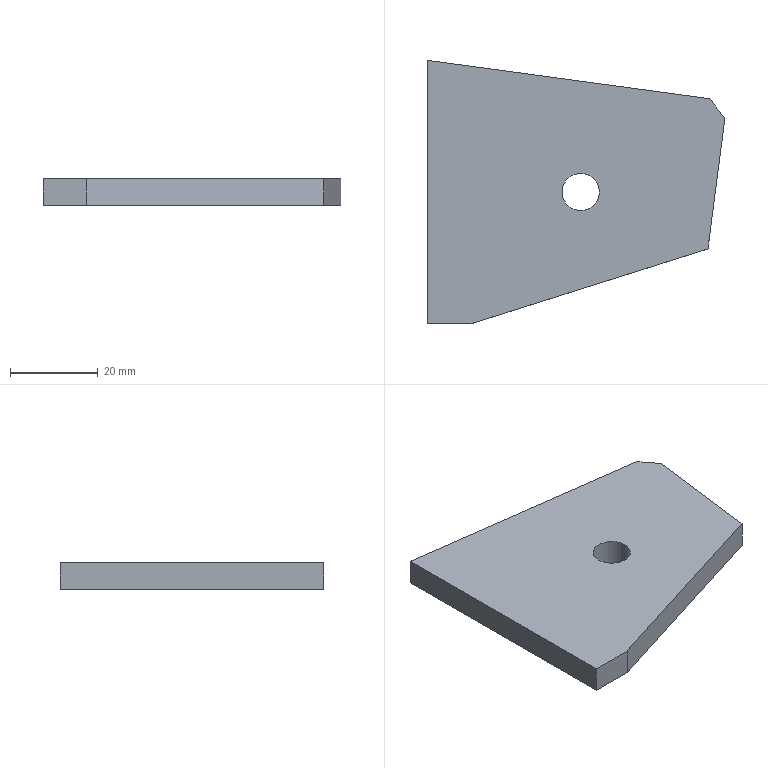Part | SolidWorks | features Chamfer 1, Extrusion 1, HoleWzd 1 | 1 solid | 10 faces | box 67.858 x 60 x 6 mm | volume 18679 mm3 | plane 8 | cylinder 2 | commonest cylinder face diameters 8.5 x2
STEP:
#1=CARTESIAN_POINT('',(39.25,30.,0.));
#2=VERTEX_POINT('',#1);
#3=CARTESIAN_POINT('',(30.75,30.,0.));
#4=VERTEX_POINT('',#3);
#5=CARTESIAN_POINT('',(35.,30.,0.));
#6=DIRECTION('',(0.,0.,-1.));
#7=DIRECTION('',(-1.,0.,0.));
#8=AXIS2_PLACEMENT_3D('',#5,#6,#7);
#9=CIRCLE('',#8,4.25);
#10=EDGE_CURVE('',#2,#4,#9,.T.);
#11=ORIENTED_EDGE('',*,*,#10,.T.);
#12=CARTESIAN_POINT('',(30.75,30.,6.));
#13=VERTEX_POINT('',#12);
#14=CARTESIAN_POINT('',(30.75,30.,6.));
#15=DIRECTION('',(0.,0.,1.));
#16=VECTOR('',#15,1000.);
#17=LINE('',#14,#16);
#18=EDGE_CURVE('',#4,#13,#17,.T.);
#19=ORIENTED_EDGE('',*,*,#18,.T.);
#20=CARTESIAN_POINT('',(39.25,30.,6.));
#21=VERTEX_POINT('',#20);
#22=CARTESIAN_POINT('',(35.,30.,6.));
#23=DIRECTION('',(0.,0.,1.));
#24=DIRECTION('',(1.,0.,0.));
#25=AXIS2_PLACEMENT_3D('',#22,#23,#24);
#26=CIRCLE('',#25,4.25);
#27=EDGE_CURVE('',#13,#21,#26,.T.);
#28=ORIENTED_EDGE('',*,*,#27,.T.);
#29=CARTESIAN_POINT('',(39.25,30.,6.));
#30=DIRECTION('',(0.,0.,1.));
#31=VECTOR('',#30,1000.);
#32=LINE('',#29,#31);
#33=EDGE_CURVE('',#2,#21,#32,.T.);
#34=ORIENTED_EDGE('',*,*,#33,.F.);
#35=EDGE_LOOP('',(#11,#19,#28,#34));
#36=FACE_OUTER_BOUND('',#35,.T.);
#37=CARTESIAN_POINT('',(35.,30.,6.));
#38=DIRECTION('',(0.,0.,1.));
#39=DIRECTION('',(1.,0.,0.));
#40=AXIS2_PLACEMENT_3D('',#37,#38,#39);
#41=CYLINDRICAL_SURFACE('',#40,4.25);
#42=ADVANCED_FACE('',(#36),#41,.F.);
#43=CARTESIAN_POINT('',(0.,60.,6.));
#44=VERTEX_POINT('',#43);
#45=CARTESIAN_POINT('',(64.385,51.26,6.));
#46=VERTEX_POINT('',#45);
#47=CARTESIAN_POINT('',(0.,60.,6.));
#48=DIRECTION('',(0.9909,-0.1345,0.));
#49=VECTOR('',#48,1000.);
#50=LINE('',#47,#49);
#51=EDGE_CURVE('',#44,#46,#50,.T.);
#52=ORIENTED_EDGE('',*,*,#51,.T.);
#53=CARTESIAN_POINT('',(64.385,51.26,0.));
#54=VERTEX_POINT('',#53);
#55=CARTESIAN_POINT('',(64.385,51.26,6.));
#56=DIRECTION('',(0.,0.,-1.));
#57=VECTOR('',#56,1000.);
#58=LINE('',#55,#57);
#59=EDGE_CURVE('',#46,#54,#58,.T.);
#60=ORIENTED_EDGE('',*,*,#59,.T.);
#61=CARTESIAN_POINT('',(0.,60.,0.));
#62=VERTEX_POINT('',#61);
#63=CARTESIAN_POINT('',(0.,60.,0.));
#64=DIRECTION('',(0.9909,-0.1345,0.));
#65=VECTOR('',#64,1000.);
#66=LINE('',#63,#65);
#67=EDGE_CURVE('',#62,#54,#66,.T.);
#68=ORIENTED_EDGE('',*,*,#67,.F.);
#69=CARTESIAN_POINT('',(0.,60.,6.));
#70=DIRECTION('',(0.,0.,-1.));
#71=VECTOR('',#70,1000.);
#72=LINE('',#69,#71);
#73=EDGE_CURVE('',#44,#62,#72,.T.);
#74=ORIENTED_EDGE('',*,*,#73,.F.);
#75=EDGE_LOOP('',(#52,#60,#68,#74));
#76=FACE_OUTER_BOUND('',#75,.T.);
#77=CARTESIAN_POINT('',(0.,60.,6.));
#78=DIRECTION('',(0.1345,0.9909,0.));
#79=DIRECTION('',(-0.9909,0.1345,0.));
#80=AXIS2_PLACEMENT_3D('',#77,#78,#79);
#81=PLANE('',#80);
#82=ADVANCED_FACE('',(#76),#81,.T.);
#83=CARTESIAN_POINT('',(0.,0.,0.));
#84=VERTEX_POINT('',#83);
#85=CARTESIAN_POINT('',(0.,0.,0.));
#86=DIRECTION('',(0.,1.,0.));
#87=VECTOR('',#86,1000.);
#88=LINE('',#85,#87);
#89=EDGE_CURVE('',#84,#62,#88,.T.);
#90=ORIENTED_EDGE('',*,*,#89,.F.);
#91=CARTESIAN_POINT('',(0.,0.,6.));
#92=VERTEX_POINT('',#91);
#93=CARTESIAN_POINT('',(0.,0.,6.));
#94=DIRECTION('',(0.,0.,-1.));
#95=VECTOR('',#94,1000.);
#96=LINE('',#93,#95);
#97=EDGE_CURVE('',#92,#84,#96,.T.);
#98=ORIENTED_EDGE('',*,*,#97,.F.);
#99=CARTESIAN_POINT('',(0.,0.,6.));
#100=DIRECTION('',(0.,1.,0.));
#101=VECTOR('',#100,1000.);
#102=LINE('',#99,#101);
#103=EDGE_CURVE('',#92,#44,#102,.T.);
#104=ORIENTED_EDGE('',*,*,#103,.T.);
#105=ORIENTED_EDGE('',*,*,#73,.T.);
#106=EDGE_LOOP('',(#90,#98,#104,#105));
#107=FACE_OUTER_BOUND('',#106,.T.);
#108=CARTESIAN_POINT('',(0.,0.,6.));
#109=DIRECTION('',(-1.,0.,0.));
#110=DIRECTION('',(0.,0.,1.));
#111=AXIS2_PLACEMENT_3D('',#108,#109,#110);
#112=PLANE('',#111);
#113=ADVANCED_FACE('',(#107),#112,.T.);
#114=CARTESIAN_POINT('',(10.,0.,0.));
#115=VERTEX_POINT('',#114);
#116=CARTESIAN_POINT('',(10.,0.,0.));
#117=DIRECTION('',(-1.,0.,0.));
#118=VECTOR('',#117,1000.);
#119=LINE('',#116,#118);
#120=EDGE_CURVE('',#115,#84,#119,.T.);
#121=ORIENTED_EDGE('',*,*,#120,.F.);
#122=CARTESIAN_POINT('',(10.,0.,6.));
#123=VERTEX_POINT('',#122);
#124=CARTESIAN_POINT('',(10.,0.,6.));
#125=DIRECTION('',(0.,0.,-1.));
#126=VECTOR('',#125,1000.);
#127=LINE('',#124,#126);
#128=EDGE_CURVE('',#123,#115,#127,.T.);
#129=ORIENTED_EDGE('',*,*,#128,.F.);
#130=CARTESIAN_POINT('',(10.,0.,6.));
#131=DIRECTION('',(-1.,0.,0.));
#132=VECTOR('',#131,1000.);
#133=LINE('',#130,#132);
#134=EDGE_CURVE('',#123,#92,#133,.T.);
#135=ORIENTED_EDGE('',*,*,#134,.T.);
#136=ORIENTED_EDGE('',*,*,#97,.T.);
#137=EDGE_LOOP('',(#121,#129,#135,#136));
#138=FACE_OUTER_BOUND('',#137,.T.);
#139=CARTESIAN_POINT('',(10.,0.,6.));
#140=DIRECTION('',(0.,-1.,0.));
#141=DIRECTION('',(1.,0.,0.));
#142=AXIS2_PLACEMENT_3D('',#139,#140,#141);
#143=PLANE('',#142);
#144=ADVANCED_FACE('',(#138),#143,.T.);
#145=CARTESIAN_POINT('',(64.,17.,0.));
#146=VERTEX_POINT('',#145);
#147=CARTESIAN_POINT('',(64.,17.,0.));
#148=DIRECTION('',(-0.9538,-0.3003,0.));
#149=VECTOR('',#148,1000.);
#150=LINE('',#147,#149);
#151=EDGE_CURVE('',#146,#115,#150,.T.);
#152=ORIENTED_EDGE('',*,*,#151,.F.);
#153=CARTESIAN_POINT('',(64.,17.,6.));
#154=VERTEX_POINT('',#153);
#155=CARTESIAN_POINT('',(64.,17.,6.));
#156=DIRECTION('',(0.,0.,-1.));
#157=VECTOR('',#156,1000.);
#158=LINE('',#155,#157);
#159=EDGE_CURVE('',#154,#146,#158,.T.);
#160=ORIENTED_EDGE('',*,*,#159,.F.);
#161=CARTESIAN_POINT('',(64.,17.,6.));
#162=DIRECTION('',(-0.9538,-0.3003,0.));
#163=VECTOR('',#162,1000.);
#164=LINE('',#161,#163);
#165=EDGE_CURVE('',#154,#123,#164,.T.);
#166=ORIENTED_EDGE('',*,*,#165,.T.);
#167=ORIENTED_EDGE('',*,*,#128,.T.);
#168=EDGE_LOOP('',(#152,#160,#166,#167));
#169=FACE_OUTER_BOUND('',#168,.T.);
#170=CARTESIAN_POINT('',(64.,17.,6.));
#171=DIRECTION('',(0.3003,-0.9538,0.));
#172=DIRECTION('',(0.9538,0.3003,0.));
#173=AXIS2_PLACEMENT_3D('',#170,#171,#172);
#174=PLANE('',#173);
#175=ADVANCED_FACE('',(#169),#174,.T.);
#176=CARTESIAN_POINT('',(67.858,46.751,0.));
#177=VERTEX_POINT('',#176);
#178=CARTESIAN_POINT('',(68.373,50.718,0.));
#179=DIRECTION('',(-0.1286,-0.9917,0.));
#180=VECTOR('',#179,1000.);
#181=LINE('',#178,#180);
#182=EDGE_CURVE('',#177,#146,#181,.T.);
#183=ORIENTED_EDGE('',*,*,#182,.F.);
#184=CARTESIAN_POINT('',(67.858,46.751,6.));
#185=VERTEX_POINT('',#184);
#186=CARTESIAN_POINT('',(67.858,46.751,6.));
#187=DIRECTION('',(0.,0.,1.));
#188=VECTOR('',#187,1000.);
#189=LINE('',#186,#188);
#190=EDGE_CURVE('',#177,#185,#189,.T.);
#191=ORIENTED_EDGE('',*,*,#190,.T.);
#192=CARTESIAN_POINT('',(68.373,50.718,6.));
#193=DIRECTION('',(-0.1286,-0.9917,0.));
#194=VECTOR('',#193,1000.);
#195=LINE('',#192,#194);
#196=EDGE_CURVE('',#185,#154,#195,.T.);
#197=ORIENTED_EDGE('',*,*,#196,.T.);
#198=ORIENTED_EDGE('',*,*,#159,.T.);
#199=EDGE_LOOP('',(#183,#191,#197,#198));
#200=FACE_OUTER_BOUND('',#199,.T.);
#201=CARTESIAN_POINT('',(68.373,50.718,6.));
#202=DIRECTION('',(0.9917,-0.1286,0.));
#203=DIRECTION('',(0.1286,0.9917,0.));
#204=AXIS2_PLACEMENT_3D('',#201,#202,#203);
#205=PLANE('',#204);
#206=ADVANCED_FACE('',(#200),#205,.T.);
#207=CARTESIAN_POINT('',(35.,30.,6.));
#208=DIRECTION('',(0.,0.,1.));
#209=DIRECTION('',(1.,0.,0.));
#210=AXIS2_PLACEMENT_3D('',#207,#208,#209);
#211=CIRCLE('',#210,4.25);
#212=EDGE_CURVE('',#21,#13,#211,.T.);
#213=ORIENTED_EDGE('',*,*,#212,.F.);
#214=ORIENTED_EDGE('',*,*,#27,.F.);
#215=EDGE_LOOP('',(#213,#214));
#216=FACE_BOUND('',#215,.T.);
#217=ORIENTED_EDGE('',*,*,#196,.F.);
#218=CARTESIAN_POINT('',(64.385,51.26,6.));
#219=DIRECTION('',(-0.6103,0.7922,0.));
#220=VECTOR('',#219,1000.);
#221=LINE('',#218,#220);
#222=EDGE_CURVE('',#185,#46,#221,.T.);
#223=ORIENTED_EDGE('',*,*,#222,.T.);
#224=ORIENTED_EDGE('',*,*,#51,.F.);
#225=ORIENTED_EDGE('',*,*,#103,.F.);
#226=ORIENTED_EDGE('',*,*,#134,.F.);
#227=ORIENTED_EDGE('',*,*,#165,.F.);
#228=EDGE_LOOP('',(#217,#223,#224,#225,#226,#227));
#229=FACE_OUTER_BOUND('',#228,.T.);
#230=CARTESIAN_POINT('',(0.,0.,6.));
#231=DIRECTION('',(0.,0.,-1.));
#232=DIRECTION('',(-1.,0.,0.));
#233=AXIS2_PLACEMENT_3D('',#230,#231,#232);
#234=PLANE('',#233);
#235=ADVANCED_FACE('',(#216,#229),#234,.F.);
#236=ORIENTED_EDGE('',*,*,#10,.F.);
#237=CARTESIAN_POINT('',(35.,30.,0.));
#238=DIRECTION('',(0.,0.,-1.));
#239=DIRECTION('',(-1.,0.,0.));
#240=AXIS2_PLACEMENT_3D('',#237,#238,#239);
#241=CIRCLE('',#240,4.25);
#242=EDGE_CURVE('',#4,#2,#241,.T.);
#243=ORIENTED_EDGE('',*,*,#242,.F.);
#244=EDGE_LOOP('',(#236,#243));
#245=FACE_BOUND('',#244,.T.);
#246=ORIENTED_EDGE('',*,*,#67,.T.);
#247=CARTESIAN_POINT('',(65.187,50.22,0.));
#248=DIRECTION('',(0.6103,-0.7922,0.));
#249=VECTOR('',#248,1000.);
#250=LINE('',#247,#249);
#251=EDGE_CURVE('',#54,#177,#250,.T.);
#252=ORIENTED_EDGE('',*,*,#251,.T.);
#253=ORIENTED_EDGE('',*,*,#182,.T.);
#254=ORIENTED_EDGE('',*,*,#151,.T.);
#255=ORIENTED_EDGE('',*,*,#120,.T.);
#256=ORIENTED_EDGE('',*,*,#89,.T.);
#257=EDGE_LOOP('',(#246,#252,#253,#254,#255,#256));
#258=FACE_OUTER_BOUND('',#257,.T.);
#259=CARTESIAN_POINT('',(0.,0.,0.));
#260=DIRECTION('',(0.,0.,-1.));
#261=DIRECTION('',(-1.,0.,0.));
#262=AXIS2_PLACEMENT_3D('',#259,#260,#261);
#263=PLANE('',#262);
#264=ADVANCED_FACE('',(#245,#258),#263,.T.);
#265=ORIENTED_EDGE('',*,*,#18,.F.);
#266=ORIENTED_EDGE('',*,*,#242,.T.);
#267=ORIENTED_EDGE('',*,*,#33,.T.);
#268=ORIENTED_EDGE('',*,*,#212,.T.);
#269=EDGE_LOOP('',(#265,#266,#267,#268));
#270=FACE_OUTER_BOUND('',#269,.T.);
#271=CARTESIAN_POINT('',(35.,30.,6.));
#272=DIRECTION('',(0.,0.,1.));
#273=DIRECTION('',(1.,0.,0.));
#274=AXIS2_PLACEMENT_3D('',#271,#272,#273);
#275=CYLINDRICAL_SURFACE('',#274,4.25);
#276=ADVANCED_FACE('',(#270),#275,.F.);
#277=ORIENTED_EDGE('',*,*,#222,.F.);
#278=ORIENTED_EDGE('',*,*,#190,.F.);
#279=ORIENTED_EDGE('',*,*,#251,.F.);
#280=ORIENTED_EDGE('',*,*,#59,.F.);
#281=EDGE_LOOP('',(#277,#278,#279,#280));
#282=FACE_OUTER_BOUND('',#281,.T.);
#283=CARTESIAN_POINT('',(64.385,51.26,6.));
#284=DIRECTION('',(-0.7922,-0.6103,0.));
#285=DIRECTION('',(0.,0.,-1.));
#286=AXIS2_PLACEMENT_3D('',#283,#284,#285);
#287=PLANE('',#286);
#288=ADVANCED_FACE('',(#282),#287,.F.);
#289=CLOSED_SHELL('',(#42,#82,#113,#144,#175,#206,#235,#264,#276,#288));
#290=MANIFOLD_SOLID_BREP('',#289);
#291=CARTESIAN_POINT('',(0.,0.,0.));
#292=DIRECTION('',(0.,0.,1.));
#293=DIRECTION('',(1.,0.,0.));
#294=AXIS2_PLACEMENT_3D('',#291,#292,#293);
#295=(LENGTH_UNIT()NAMED_UNIT(*)SI_UNIT(.MILLI.,.METRE.));
#296=UNCERTAINTY_MEASURE_WITH_UNIT(LENGTH_MEASURE(0.00001),#295,'','');
#297=(NAMED_UNIT(*)PLANE_ANGLE_UNIT()SI_UNIT($,.RADIAN.));
#298=(NAMED_UNIT(*)SI_UNIT($,.STERADIAN.)SOLID_ANGLE_UNIT());
#299=(GEOMETRIC_REPRESENTATION_CONTEXT(3)GLOBAL_UNCERTAINTY_ASSIGNED_CONTEXT((#296))GLOBAL_UNIT_ASSIGNED_CONTEXT((#295,#297,#298))REPRESENTATION_CONTEXT('',''));
#300=ADVANCED_BREP_SHAPE_REPRESENTATION('',(#290,#294),#299);